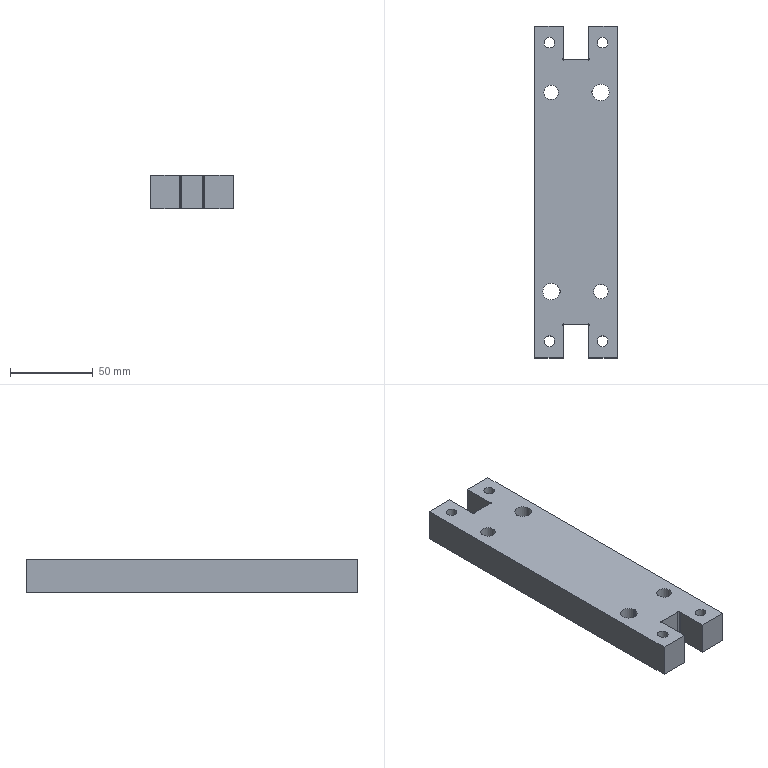Part | STEP file | YBQDJ-DX-1 | 1 solid | 48 faces | box 50 x 200 x 20 mm | volume 177964 mm3 | cylinder 30 | plane 18 | commonest cylinder face diameters 2 x8 1 x6 4 x4 6.5 x4 11 x4 8.7 x2